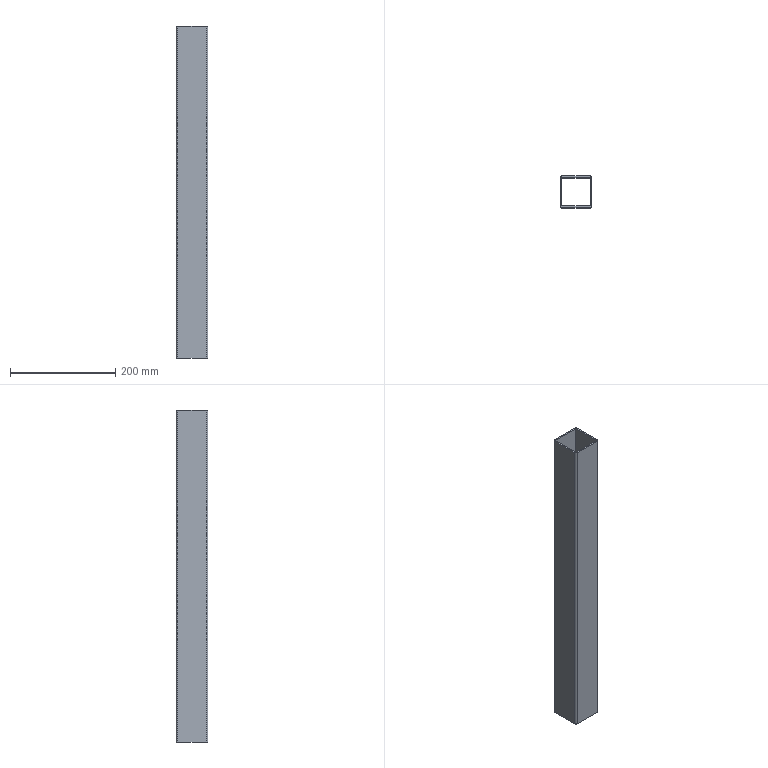Part | STEP file | X77-03105 | 1 solid | 14 faces | box 60 x 60 x 630 mm | volume 426053 mm3 | plane 10 | cylinder 4 | commonest cylinder face diameters 6 x4
STEP:
#1=CARTESIAN_POINT('',(0.,3.,630.));
#2=VERTEX_POINT('',#1);
#3=CARTESIAN_POINT('',(3.,0.,630.));
#4=VERTEX_POINT('',#3);
#5=CARTESIAN_POINT('',(3.,3.,630.));
#6=DIRECTION('',(0.,0.,1.));
#7=DIRECTION('',(1.,0.,0.));
#8=AXIS2_PLACEMENT_3D('',#5,#6,#7);
#9=CIRCLE('',#8,3.);
#10=EDGE_CURVE('',#2,#4,#9,.T.);
#11=ORIENTED_EDGE('',*,*,#10,.T.);
#12=CARTESIAN_POINT('',(57.,0.,630.));
#13=VERTEX_POINT('',#12);
#14=CARTESIAN_POINT('',(3.,0.,630.));
#15=DIRECTION('',(1.,0.,0.));
#16=VECTOR('',#15,1000.);
#17=LINE('',#14,#16);
#18=EDGE_CURVE('',#4,#13,#17,.T.);
#19=ORIENTED_EDGE('',*,*,#18,.T.);
#20=CARTESIAN_POINT('',(60.,3.,630.));
#21=VERTEX_POINT('',#20);
#22=CARTESIAN_POINT('',(57.,3.,630.));
#23=DIRECTION('',(0.,0.,1.));
#24=DIRECTION('',(1.,0.,0.));
#25=AXIS2_PLACEMENT_3D('',#22,#23,#24);
#26=CIRCLE('',#25,3.);
#27=EDGE_CURVE('',#13,#21,#26,.T.);
#28=ORIENTED_EDGE('',*,*,#27,.T.);
#29=CARTESIAN_POINT('',(60.,57.,630.));
#30=VERTEX_POINT('',#29);
#31=CARTESIAN_POINT('',(60.,3.,630.));
#32=DIRECTION('',(0.,1.,0.));
#33=VECTOR('',#32,1000.);
#34=LINE('',#31,#33);
#35=EDGE_CURVE('',#21,#30,#34,.T.);
#36=ORIENTED_EDGE('',*,*,#35,.T.);
#37=CARTESIAN_POINT('',(57.,60.,630.));
#38=VERTEX_POINT('',#37);
#39=CARTESIAN_POINT('',(57.,57.,630.));
#40=DIRECTION('',(0.,0.,1.));
#41=DIRECTION('',(1.,0.,0.));
#42=AXIS2_PLACEMENT_3D('',#39,#40,#41);
#43=CIRCLE('',#42,3.);
#44=EDGE_CURVE('',#30,#38,#43,.T.);
#45=ORIENTED_EDGE('',*,*,#44,.T.);
#46=CARTESIAN_POINT('',(3.,60.,630.));
#47=VERTEX_POINT('',#46);
#48=CARTESIAN_POINT('',(3.,60.,630.));
#49=DIRECTION('',(-1.,0.,0.));
#50=VECTOR('',#49,1000.);
#51=LINE('',#48,#50);
#52=EDGE_CURVE('',#38,#47,#51,.T.);
#53=ORIENTED_EDGE('',*,*,#52,.T.);
#54=CARTESIAN_POINT('',(0.,57.,630.));
#55=VERTEX_POINT('',#54);
#56=CARTESIAN_POINT('',(3.,57.,630.));
#57=DIRECTION('',(0.,0.,1.));
#58=DIRECTION('',(1.,0.,0.));
#59=AXIS2_PLACEMENT_3D('',#56,#57,#58);
#60=CIRCLE('',#59,3.);
#61=EDGE_CURVE('',#47,#55,#60,.T.);
#62=ORIENTED_EDGE('',*,*,#61,.T.);
#63=CARTESIAN_POINT('',(0.,3.,630.));
#64=DIRECTION('',(0.,-1.,0.));
#65=VECTOR('',#64,1000.);
#66=LINE('',#63,#65);
#67=EDGE_CURVE('',#55,#2,#66,.T.);
#68=ORIENTED_EDGE('',*,*,#67,.T.);
#69=EDGE_LOOP('',(#11,#19,#28,#36,#45,#53,#62,#68));
#70=FACE_OUTER_BOUND('',#69,.T.);
#71=CARTESIAN_POINT('',(3.,3.,630.));
#72=VERTEX_POINT('',#71);
#73=CARTESIAN_POINT('',(57.,3.,630.));
#74=VERTEX_POINT('',#73);
#75=CARTESIAN_POINT('',(3.,3.,630.));
#76=DIRECTION('',(1.,0.,0.));
#77=VECTOR('',#76,1000.);
#78=LINE('',#75,#77);
#79=EDGE_CURVE('',#72,#74,#78,.T.);
#80=ORIENTED_EDGE('',*,*,#79,.F.);
#81=CARTESIAN_POINT('',(3.,57.,630.));
#82=VERTEX_POINT('',#81);
#83=CARTESIAN_POINT('',(3.,3.,630.));
#84=DIRECTION('',(0.,-1.,0.));
#85=VECTOR('',#84,1000.);
#86=LINE('',#83,#85);
#87=EDGE_CURVE('',#82,#72,#86,.T.);
#88=ORIENTED_EDGE('',*,*,#87,.F.);
#89=CARTESIAN_POINT('',(57.,57.,630.));
#90=VERTEX_POINT('',#89);
#91=CARTESIAN_POINT('',(3.,57.,630.));
#92=DIRECTION('',(-1.,0.,0.));
#93=VECTOR('',#92,1000.);
#94=LINE('',#91,#93);
#95=EDGE_CURVE('',#90,#82,#94,.T.);
#96=ORIENTED_EDGE('',*,*,#95,.F.);
#97=CARTESIAN_POINT('',(57.,3.,630.));
#98=DIRECTION('',(0.,1.,0.));
#99=VECTOR('',#98,1000.);
#100=LINE('',#97,#99);
#101=EDGE_CURVE('',#74,#90,#100,.T.);
#102=ORIENTED_EDGE('',*,*,#101,.F.);
#103=EDGE_LOOP('',(#80,#88,#96,#102));
#104=FACE_BOUND('',#103,.T.);
#105=CARTESIAN_POINT('',(3.,3.,630.));
#106=DIRECTION('',(0.,0.,1.));
#107=DIRECTION('',(1.,0.,0.));
#108=AXIS2_PLACEMENT_3D('',#105,#106,#107);
#109=PLANE('',#108);
#110=ADVANCED_FACE('',(#70,#104),#109,.T.);
#111=CARTESIAN_POINT('',(0.,3.,0.));
#112=VERTEX_POINT('',#111);
#113=CARTESIAN_POINT('',(3.,0.,0.));
#114=VERTEX_POINT('',#113);
#115=CARTESIAN_POINT('',(3.,3.,0.));
#116=DIRECTION('',(0.,0.,1.));
#117=DIRECTION('',(1.,0.,0.));
#118=AXIS2_PLACEMENT_3D('',#115,#116,#117);
#119=CIRCLE('',#118,3.);
#120=EDGE_CURVE('',#112,#114,#119,.T.);
#121=ORIENTED_EDGE('',*,*,#120,.F.);
#122=CARTESIAN_POINT('',(0.,57.,0.));
#123=VERTEX_POINT('',#122);
#124=CARTESIAN_POINT('',(0.,3.,0.));
#125=DIRECTION('',(0.,-1.,0.));
#126=VECTOR('',#125,1000.);
#127=LINE('',#124,#126);
#128=EDGE_CURVE('',#123,#112,#127,.T.);
#129=ORIENTED_EDGE('',*,*,#128,.F.);
#130=CARTESIAN_POINT('',(3.,60.,0.));
#131=VERTEX_POINT('',#130);
#132=CARTESIAN_POINT('',(3.,57.,0.));
#133=DIRECTION('',(0.,0.,1.));
#134=DIRECTION('',(1.,0.,0.));
#135=AXIS2_PLACEMENT_3D('',#132,#133,#134);
#136=CIRCLE('',#135,3.);
#137=EDGE_CURVE('',#131,#123,#136,.T.);
#138=ORIENTED_EDGE('',*,*,#137,.F.);
#139=CARTESIAN_POINT('',(57.,60.,0.));
#140=VERTEX_POINT('',#139);
#141=CARTESIAN_POINT('',(3.,60.,0.));
#142=DIRECTION('',(-1.,0.,0.));
#143=VECTOR('',#142,1000.);
#144=LINE('',#141,#143);
#145=EDGE_CURVE('',#140,#131,#144,.T.);
#146=ORIENTED_EDGE('',*,*,#145,.F.);
#147=CARTESIAN_POINT('',(60.,57.,0.));
#148=VERTEX_POINT('',#147);
#149=CARTESIAN_POINT('',(57.,57.,0.));
#150=DIRECTION('',(0.,0.,1.));
#151=DIRECTION('',(1.,0.,0.));
#152=AXIS2_PLACEMENT_3D('',#149,#150,#151);
#153=CIRCLE('',#152,3.);
#154=EDGE_CURVE('',#148,#140,#153,.T.);
#155=ORIENTED_EDGE('',*,*,#154,.F.);
#156=CARTESIAN_POINT('',(60.,3.,0.));
#157=VERTEX_POINT('',#156);
#158=CARTESIAN_POINT('',(60.,3.,0.));
#159=DIRECTION('',(0.,1.,0.));
#160=VECTOR('',#159,1000.);
#161=LINE('',#158,#160);
#162=EDGE_CURVE('',#157,#148,#161,.T.);
#163=ORIENTED_EDGE('',*,*,#162,.F.);
#164=CARTESIAN_POINT('',(57.,0.,0.));
#165=VERTEX_POINT('',#164);
#166=CARTESIAN_POINT('',(57.,3.,0.));
#167=DIRECTION('',(0.,0.,1.));
#168=DIRECTION('',(1.,0.,0.));
#169=AXIS2_PLACEMENT_3D('',#166,#167,#168);
#170=CIRCLE('',#169,3.);
#171=EDGE_CURVE('',#165,#157,#170,.T.);
#172=ORIENTED_EDGE('',*,*,#171,.F.);
#173=CARTESIAN_POINT('',(3.,0.,0.));
#174=DIRECTION('',(1.,0.,0.));
#175=VECTOR('',#174,1000.);
#176=LINE('',#173,#175);
#177=EDGE_CURVE('',#114,#165,#176,.T.);
#178=ORIENTED_EDGE('',*,*,#177,.F.);
#179=EDGE_LOOP('',(#121,#129,#138,#146,#155,#163,#172,#178));
#180=FACE_OUTER_BOUND('',#179,.T.);
#181=CARTESIAN_POINT('',(3.,57.,0.));
#182=VERTEX_POINT('',#181);
#183=CARTESIAN_POINT('',(3.,3.,0.));
#184=VERTEX_POINT('',#183);
#185=CARTESIAN_POINT('',(3.,3.,0.));
#186=DIRECTION('',(0.,-1.,0.));
#187=VECTOR('',#186,1000.);
#188=LINE('',#185,#187);
#189=EDGE_CURVE('',#182,#184,#188,.T.);
#190=ORIENTED_EDGE('',*,*,#189,.T.);
#191=CARTESIAN_POINT('',(57.,3.,0.));
#192=VERTEX_POINT('',#191);
#193=CARTESIAN_POINT('',(3.,3.,0.));
#194=DIRECTION('',(1.,0.,0.));
#195=VECTOR('',#194,1000.);
#196=LINE('',#193,#195);
#197=EDGE_CURVE('',#184,#192,#196,.T.);
#198=ORIENTED_EDGE('',*,*,#197,.T.);
#199=CARTESIAN_POINT('',(57.,57.,0.));
#200=VERTEX_POINT('',#199);
#201=CARTESIAN_POINT('',(57.,3.,0.));
#202=DIRECTION('',(0.,1.,0.));
#203=VECTOR('',#202,1000.);
#204=LINE('',#201,#203);
#205=EDGE_CURVE('',#192,#200,#204,.T.);
#206=ORIENTED_EDGE('',*,*,#205,.T.);
#207=CARTESIAN_POINT('',(3.,57.,0.));
#208=DIRECTION('',(-1.,0.,0.));
#209=VECTOR('',#208,1000.);
#210=LINE('',#207,#209);
#211=EDGE_CURVE('',#200,#182,#210,.T.);
#212=ORIENTED_EDGE('',*,*,#211,.T.);
#213=EDGE_LOOP('',(#190,#198,#206,#212));
#214=FACE_BOUND('',#213,.T.);
#215=CARTESIAN_POINT('',(3.,3.,0.));
#216=DIRECTION('',(0.,0.,1.));
#217=DIRECTION('',(1.,0.,0.));
#218=AXIS2_PLACEMENT_3D('',#215,#216,#217);
#219=PLANE('',#218);
#220=ADVANCED_FACE('',(#180,#214),#219,.F.);
#221=ORIENTED_EDGE('',*,*,#120,.T.);
#222=CARTESIAN_POINT('',(3.,0.,630.));
#223=DIRECTION('',(0.,0.,-1.));
#224=VECTOR('',#223,1000.);
#225=LINE('',#222,#224);
#226=EDGE_CURVE('',#4,#114,#225,.T.);
#227=ORIENTED_EDGE('',*,*,#226,.F.);
#228=ORIENTED_EDGE('',*,*,#10,.F.);
#229=CARTESIAN_POINT('',(0.,3.,630.));
#230=DIRECTION('',(0.,0.,-1.));
#231=VECTOR('',#230,1000.);
#232=LINE('',#229,#231);
#233=EDGE_CURVE('',#2,#112,#232,.T.);
#234=ORIENTED_EDGE('',*,*,#233,.T.);
#235=EDGE_LOOP('',(#221,#227,#228,#234));
#236=FACE_OUTER_BOUND('',#235,.T.);
#237=CARTESIAN_POINT('',(3.,3.,630.));
#238=DIRECTION('',(0.,0.,-1.));
#239=DIRECTION('',(-1.,0.,0.));
#240=AXIS2_PLACEMENT_3D('',#237,#238,#239);
#241=CYLINDRICAL_SURFACE('',#240,3.);
#242=ADVANCED_FACE('',(#236),#241,.T.);
#243=ORIENTED_EDGE('',*,*,#177,.T.);
#244=CARTESIAN_POINT('',(57.,0.,630.));
#245=DIRECTION('',(0.,0.,-1.));
#246=VECTOR('',#245,1000.);
#247=LINE('',#244,#246);
#248=EDGE_CURVE('',#13,#165,#247,.T.);
#249=ORIENTED_EDGE('',*,*,#248,.F.);
#250=ORIENTED_EDGE('',*,*,#18,.F.);
#251=ORIENTED_EDGE('',*,*,#226,.T.);
#252=EDGE_LOOP('',(#243,#249,#250,#251));
#253=FACE_OUTER_BOUND('',#252,.T.);
#254=CARTESIAN_POINT('',(3.,0.,630.));
#255=DIRECTION('',(0.,1.,0.));
#256=DIRECTION('',(0.,0.,1.));
#257=AXIS2_PLACEMENT_3D('',#254,#255,#256);
#258=PLANE('',#257);
#259=ADVANCED_FACE('',(#253),#258,.F.);
#260=ORIENTED_EDGE('',*,*,#171,.T.);
#261=CARTESIAN_POINT('',(60.,3.,630.));
#262=DIRECTION('',(0.,0.,-1.));
#263=VECTOR('',#262,1000.);
#264=LINE('',#261,#263);
#265=EDGE_CURVE('',#21,#157,#264,.T.);
#266=ORIENTED_EDGE('',*,*,#265,.F.);
#267=ORIENTED_EDGE('',*,*,#27,.F.);
#268=ORIENTED_EDGE('',*,*,#248,.T.);
#269=EDGE_LOOP('',(#260,#266,#267,#268));
#270=FACE_OUTER_BOUND('',#269,.T.);
#271=CARTESIAN_POINT('',(57.,3.,630.));
#272=DIRECTION('',(0.,0.,-1.));
#273=DIRECTION('',(-1.,0.,0.));
#274=AXIS2_PLACEMENT_3D('',#271,#272,#273);
#275=CYLINDRICAL_SURFACE('',#274,3.);
#276=ADVANCED_FACE('',(#270),#275,.T.);
#277=ORIENTED_EDGE('',*,*,#162,.T.);
#278=CARTESIAN_POINT('',(60.,57.,630.));
#279=DIRECTION('',(0.,0.,-1.));
#280=VECTOR('',#279,1000.);
#281=LINE('',#278,#280);
#282=EDGE_CURVE('',#30,#148,#281,.T.);
#283=ORIENTED_EDGE('',*,*,#282,.F.);
#284=ORIENTED_EDGE('',*,*,#35,.F.);
#285=ORIENTED_EDGE('',*,*,#265,.T.);
#286=EDGE_LOOP('',(#277,#283,#284,#285));
#287=FACE_OUTER_BOUND('',#286,.T.);
#288=CARTESIAN_POINT('',(60.,3.,630.));
#289=DIRECTION('',(-1.,0.,0.));
#290=DIRECTION('',(0.,0.,1.));
#291=AXIS2_PLACEMENT_3D('',#288,#289,#290);
#292=PLANE('',#291);
#293=ADVANCED_FACE('',(#287),#292,.F.);
#294=ORIENTED_EDGE('',*,*,#154,.T.);
#295=CARTESIAN_POINT('',(57.,60.,630.));
#296=DIRECTION('',(0.,0.,-1.));
#297=VECTOR('',#296,1000.);
#298=LINE('',#295,#297);
#299=EDGE_CURVE('',#38,#140,#298,.T.);
#300=ORIENTED_EDGE('',*,*,#299,.F.);
#301=ORIENTED_EDGE('',*,*,#44,.F.);
#302=ORIENTED_EDGE('',*,*,#282,.T.);
#303=EDGE_LOOP('',(#294,#300,#301,#302));
#304=FACE_OUTER_BOUND('',#303,.T.);
#305=CARTESIAN_POINT('',(57.,57.,630.));
#306=DIRECTION('',(0.,0.,-1.));
#307=DIRECTION('',(-1.,0.,0.));
#308=AXIS2_PLACEMENT_3D('',#305,#306,#307);
#309=CYLINDRICAL_SURFACE('',#308,3.);
#310=ADVANCED_FACE('',(#304),#309,.T.);
#311=ORIENTED_EDGE('',*,*,#145,.T.);
#312=CARTESIAN_POINT('',(3.,60.,630.));
#313=DIRECTION('',(0.,0.,-1.));
#314=VECTOR('',#313,1000.);
#315=LINE('',#312,#314);
#316=EDGE_CURVE('',#47,#131,#315,.T.);
#317=ORIENTED_EDGE('',*,*,#316,.F.);
#318=ORIENTED_EDGE('',*,*,#52,.F.);
#319=ORIENTED_EDGE('',*,*,#299,.T.);
#320=EDGE_LOOP('',(#311,#317,#318,#319));
#321=FACE_OUTER_BOUND('',#320,.T.);
#322=CARTESIAN_POINT('',(3.,60.,630.));
#323=DIRECTION('',(0.,-1.,0.));
#324=DIRECTION('',(0.,0.,-1.));
#325=AXIS2_PLACEMENT_3D('',#322,#323,#324);
#326=PLANE('',#325);
#327=ADVANCED_FACE('',(#321),#326,.F.);
#328=ORIENTED_EDGE('',*,*,#137,.T.);
#329=CARTESIAN_POINT('',(0.,57.,630.));
#330=DIRECTION('',(0.,0.,-1.));
#331=VECTOR('',#330,1000.);
#332=LINE('',#329,#331);
#333=EDGE_CURVE('',#55,#123,#332,.T.);
#334=ORIENTED_EDGE('',*,*,#333,.F.);
#335=ORIENTED_EDGE('',*,*,#61,.F.);
#336=ORIENTED_EDGE('',*,*,#316,.T.);
#337=EDGE_LOOP('',(#328,#334,#335,#336));
#338=FACE_OUTER_BOUND('',#337,.T.);
#339=CARTESIAN_POINT('',(3.,57.,630.));
#340=DIRECTION('',(0.,0.,-1.));
#341=DIRECTION('',(-1.,0.,0.));
#342=AXIS2_PLACEMENT_3D('',#339,#340,#341);
#343=CYLINDRICAL_SURFACE('',#342,3.);
#344=ADVANCED_FACE('',(#338),#343,.T.);
#345=ORIENTED_EDGE('',*,*,#128,.T.);
#346=ORIENTED_EDGE('',*,*,#233,.F.);
#347=ORIENTED_EDGE('',*,*,#67,.F.);
#348=ORIENTED_EDGE('',*,*,#333,.T.);
#349=EDGE_LOOP('',(#345,#346,#347,#348));
#350=FACE_OUTER_BOUND('',#349,.T.);
#351=CARTESIAN_POINT('',(0.,3.,630.));
#352=DIRECTION('',(1.,0.,0.));
#353=DIRECTION('',(0.,0.,-1.));
#354=AXIS2_PLACEMENT_3D('',#351,#352,#353);
#355=PLANE('',#354);
#356=ADVANCED_FACE('',(#350),#355,.F.);
#357=ORIENTED_EDGE('',*,*,#189,.F.);
#358=CARTESIAN_POINT('',(3.,57.,630.));
#359=DIRECTION('',(0.,0.,-1.));
#360=VECTOR('',#359,1000.);
#361=LINE('',#358,#360);
#362=EDGE_CURVE('',#82,#182,#361,.T.);
#363=ORIENTED_EDGE('',*,*,#362,.F.);
#364=ORIENTED_EDGE('',*,*,#87,.T.);
#365=CARTESIAN_POINT('',(3.,3.,630.));
#366=DIRECTION('',(0.,0.,-1.));
#367=VECTOR('',#366,1000.);
#368=LINE('',#365,#367);
#369=EDGE_CURVE('',#72,#184,#368,.T.);
#370=ORIENTED_EDGE('',*,*,#369,.T.);
#371=EDGE_LOOP('',(#357,#363,#364,#370));
#372=FACE_OUTER_BOUND('',#371,.T.);
#373=CARTESIAN_POINT('',(3.,3.,630.));
#374=DIRECTION('',(1.,0.,0.));
#375=DIRECTION('',(0.,0.,-1.));
#376=AXIS2_PLACEMENT_3D('',#373,#374,#375);
#377=PLANE('',#376);
#378=ADVANCED_FACE('',(#372),#377,.T.);
#379=ORIENTED_EDGE('',*,*,#197,.F.);
#380=ORIENTED_EDGE('',*,*,#369,.F.);
#381=ORIENTED_EDGE('',*,*,#79,.T.);
#382=CARTESIAN_POINT('',(57.,3.,630.));
#383=DIRECTION('',(0.,0.,-1.));
#384=VECTOR('',#383,1000.);
#385=LINE('',#382,#384);
#386=EDGE_CURVE('',#74,#192,#385,.T.);
#387=ORIENTED_EDGE('',*,*,#386,.T.);
#388=EDGE_LOOP('',(#379,#380,#381,#387));
#389=FACE_OUTER_BOUND('',#388,.T.);
#390=CARTESIAN_POINT('',(3.,3.,630.));
#391=DIRECTION('',(0.,1.,0.));
#392=DIRECTION('',(0.,0.,1.));
#393=AXIS2_PLACEMENT_3D('',#390,#391,#392);
#394=PLANE('',#393);
#395=ADVANCED_FACE('',(#389),#394,.T.);
#396=ORIENTED_EDGE('',*,*,#205,.F.);
#397=ORIENTED_EDGE('',*,*,#386,.F.);
#398=ORIENTED_EDGE('',*,*,#101,.T.);
#399=CARTESIAN_POINT('',(57.,57.,630.));
#400=DIRECTION('',(0.,0.,-1.));
#401=VECTOR('',#400,1000.);
#402=LINE('',#399,#401);
#403=EDGE_CURVE('',#90,#200,#402,.T.);
#404=ORIENTED_EDGE('',*,*,#403,.T.);
#405=EDGE_LOOP('',(#396,#397,#398,#404));
#406=FACE_OUTER_BOUND('',#405,.T.);
#407=CARTESIAN_POINT('',(57.,3.,630.));
#408=DIRECTION('',(-1.,0.,0.));
#409=DIRECTION('',(0.,0.,1.));
#410=AXIS2_PLACEMENT_3D('',#407,#408,#409);
#411=PLANE('',#410);
#412=ADVANCED_FACE('',(#406),#411,.T.);
#413=ORIENTED_EDGE('',*,*,#211,.F.);
#414=ORIENTED_EDGE('',*,*,#403,.F.);
#415=ORIENTED_EDGE('',*,*,#95,.T.);
#416=ORIENTED_EDGE('',*,*,#362,.T.);
#417=EDGE_LOOP('',(#413,#414,#415,#416));
#418=FACE_OUTER_BOUND('',#417,.T.);
#419=CARTESIAN_POINT('',(3.,57.,630.));
#420=DIRECTION('',(0.,-1.,0.));
#421=DIRECTION('',(0.,0.,-1.));
#422=AXIS2_PLACEMENT_3D('',#419,#420,#421);
#423=PLANE('',#422);
#424=ADVANCED_FACE('',(#418),#423,.T.);
#425=CLOSED_SHELL('',(#110,#220,#242,#259,#276,#293,#310,#327,#344,#356,#378,#395,#412,#424));
#426=MANIFOLD_SOLID_BREP('',#425);
#427=CARTESIAN_POINT('',(0.,0.,0.));
#428=DIRECTION('',(0.,0.,1.));
#429=DIRECTION('',(1.,0.,0.));
#430=AXIS2_PLACEMENT_3D('',#427,#428,#429);
#431=(LENGTH_UNIT()NAMED_UNIT(*)SI_UNIT(.MILLI.,.METRE.));
#432=UNCERTAINTY_MEASURE_WITH_UNIT(LENGTH_MEASURE(0.00001),#431,'','');
#433=(NAMED_UNIT(*)PLANE_ANGLE_UNIT()SI_UNIT($,.RADIAN.));
#434=(NAMED_UNIT(*)SI_UNIT($,.STERADIAN.)SOLID_ANGLE_UNIT());
#435=(GEOMETRIC_REPRESENTATION_CONTEXT(3)GLOBAL_UNCERTAINTY_ASSIGNED_CONTEXT((#432))GLOBAL_UNIT_ASSIGNED_CONTEXT((#431,#433,#434))REPRESENTATION_CONTEXT('',''));
#436=ADVANCED_BREP_SHAPE_REPRESENTATION('',(#426,#430),#435);